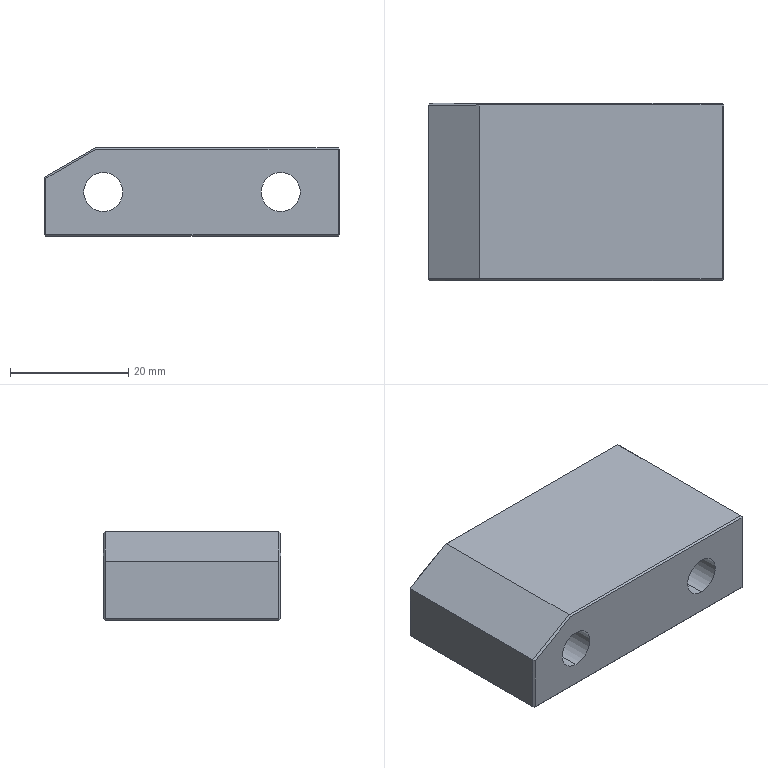Part | SolidWorks | features Chamfer 2, Extrusion 1, HoleWzd 1 | 1 solid | 36 faces | box 50 x 30 x 15 mm | volume 18955 mm3 | plane 28 | cylinder 8 | commonest cylinder face diameters 6.6 x4 11 x4
STEP:
#1=CARTESIAN_POINT('',(-15.,8.2,2.));
#2=VERTEX_POINT('',#1);
#3=CARTESIAN_POINT('',(-15.,8.2,13.));
#4=VERTEX_POINT('',#3);
#5=CARTESIAN_POINT('',(-15.,8.2,7.5));
#6=DIRECTION('',(0.,1.,0.));
#7=DIRECTION('',(0.,0.,1.));
#8=AXIS2_PLACEMENT_3D('',#5,#6,#7);
#9=CIRCLE('',#8,5.5);
#10=EDGE_CURVE('',#2,#4,#9,.T.);
#11=ORIENTED_EDGE('',*,*,#10,.F.);
#12=CARTESIAN_POINT('',(-15.,15.,2.));
#13=VERTEX_POINT('',#12);
#14=CARTESIAN_POINT('',(-15.,15.,2.));
#15=DIRECTION('',(0.,1.,0.));
#16=VECTOR('',#15,1000.);
#17=LINE('',#14,#16);
#18=EDGE_CURVE('',#2,#13,#17,.T.);
#19=ORIENTED_EDGE('',*,*,#18,.T.);
#20=CARTESIAN_POINT('',(-15.,15.,13.));
#21=VERTEX_POINT('',#20);
#22=CARTESIAN_POINT('',(-15.,15.,7.5));
#23=DIRECTION('',(0.,1.,0.));
#24=DIRECTION('',(0.,0.,1.));
#25=AXIS2_PLACEMENT_3D('',#22,#23,#24);
#26=CIRCLE('',#25,5.5);
#27=EDGE_CURVE('',#13,#21,#26,.T.);
#28=ORIENTED_EDGE('',*,*,#27,.T.);
#29=CARTESIAN_POINT('',(-15.,15.,13.));
#30=DIRECTION('',(0.,1.,0.));
#31=VECTOR('',#30,1000.);
#32=LINE('',#29,#31);
#33=EDGE_CURVE('',#4,#21,#32,.T.);
#34=ORIENTED_EDGE('',*,*,#33,.F.);
#35=EDGE_LOOP('',(#11,#19,#28,#34));
#36=FACE_OUTER_BOUND('',#35,.T.);
#37=CARTESIAN_POINT('',(-15.,15.,7.5));
#38=DIRECTION('',(0.,1.,0.));
#39=DIRECTION('',(0.,0.,1.));
#40=AXIS2_PLACEMENT_3D('',#37,#38,#39);
#41=CYLINDRICAL_SURFACE('',#40,5.5);
#42=ADVANCED_FACE('',(#36),#41,.F.);
#43=CARTESIAN_POINT('',(-15.,-15.,4.2));
#44=VERTEX_POINT('',#43);
#45=CARTESIAN_POINT('',(-15.,-15.,10.8));
#46=VERTEX_POINT('',#45);
#47=CARTESIAN_POINT('',(-15.,-15.,7.5));
#48=DIRECTION('',(0.,1.,0.));
#49=DIRECTION('',(0.,0.,1.));
#50=AXIS2_PLACEMENT_3D('',#47,#48,#49);
#51=CIRCLE('',#50,3.3);
#52=EDGE_CURVE('',#44,#46,#51,.T.);
#53=ORIENTED_EDGE('',*,*,#52,.F.);
#54=CARTESIAN_POINT('',(-15.,8.2,4.2));
#55=VERTEX_POINT('',#54);
#56=CARTESIAN_POINT('',(-15.,15.,4.2));
#57=DIRECTION('',(0.,1.,0.));
#58=VECTOR('',#57,1000.);
#59=LINE('',#56,#58);
#60=EDGE_CURVE('',#44,#55,#59,.T.);
#61=ORIENTED_EDGE('',*,*,#60,.T.);
#62=CARTESIAN_POINT('',(-15.,8.2,10.8));
#63=VERTEX_POINT('',#62);
#64=CARTESIAN_POINT('',(-15.,8.2,7.5));
#65=DIRECTION('',(0.,1.,0.));
#66=DIRECTION('',(0.,0.,1.));
#67=AXIS2_PLACEMENT_3D('',#64,#65,#66);
#68=CIRCLE('',#67,3.3);
#69=EDGE_CURVE('',#55,#63,#68,.T.);
#70=ORIENTED_EDGE('',*,*,#69,.T.);
#71=CARTESIAN_POINT('',(-15.,15.,10.8));
#72=DIRECTION('',(0.,1.,0.));
#73=VECTOR('',#72,1000.);
#74=LINE('',#71,#73);
#75=EDGE_CURVE('',#46,#63,#74,.T.);
#76=ORIENTED_EDGE('',*,*,#75,.F.);
#77=EDGE_LOOP('',(#53,#61,#70,#76));
#78=FACE_OUTER_BOUND('',#77,.T.);
#79=CARTESIAN_POINT('',(-15.,15.,7.5));
#80=DIRECTION('',(0.,1.,0.));
#81=DIRECTION('',(0.,0.,1.));
#82=AXIS2_PLACEMENT_3D('',#79,#80,#81);
#83=CYLINDRICAL_SURFACE('',#82,3.3);
#84=ADVANCED_FACE('',(#78),#83,.F.);
#85=CARTESIAN_POINT('',(15.,8.2,2.));
#86=VERTEX_POINT('',#85);
#87=CARTESIAN_POINT('',(15.,8.2,13.));
#88=VERTEX_POINT('',#87);
#89=CARTESIAN_POINT('',(15.,8.2,7.5));
#90=DIRECTION('',(0.,1.,0.));
#91=DIRECTION('',(0.,0.,1.));
#92=AXIS2_PLACEMENT_3D('',#89,#90,#91);
#93=CIRCLE('',#92,5.5);
#94=EDGE_CURVE('',#86,#88,#93,.T.);
#95=ORIENTED_EDGE('',*,*,#94,.F.);
#96=CARTESIAN_POINT('',(15.,15.,2.));
#97=VERTEX_POINT('',#96);
#98=CARTESIAN_POINT('',(15.,15.,2.));
#99=DIRECTION('',(0.,1.,0.));
#100=VECTOR('',#99,1000.);
#101=LINE('',#98,#100);
#102=EDGE_CURVE('',#86,#97,#101,.T.);
#103=ORIENTED_EDGE('',*,*,#102,.T.);
#104=CARTESIAN_POINT('',(15.,15.,13.));
#105=VERTEX_POINT('',#104);
#106=CARTESIAN_POINT('',(15.,15.,7.5));
#107=DIRECTION('',(0.,1.,0.));
#108=DIRECTION('',(0.,0.,1.));
#109=AXIS2_PLACEMENT_3D('',#106,#107,#108);
#110=CIRCLE('',#109,5.5);
#111=EDGE_CURVE('',#97,#105,#110,.T.);
#112=ORIENTED_EDGE('',*,*,#111,.T.);
#113=CARTESIAN_POINT('',(15.,15.,13.));
#114=DIRECTION('',(0.,1.,0.));
#115=VECTOR('',#114,1000.);
#116=LINE('',#113,#115);
#117=EDGE_CURVE('',#88,#105,#116,.T.);
#118=ORIENTED_EDGE('',*,*,#117,.F.);
#119=EDGE_LOOP('',(#95,#103,#112,#118));
#120=FACE_OUTER_BOUND('',#119,.T.);
#121=CARTESIAN_POINT('',(15.,15.,7.5));
#122=DIRECTION('',(0.,1.,0.));
#123=DIRECTION('',(0.,0.,1.));
#124=AXIS2_PLACEMENT_3D('',#121,#122,#123);
#125=CYLINDRICAL_SURFACE('',#124,5.5);
#126=ADVANCED_FACE('',(#120),#125,.F.);
#127=CARTESIAN_POINT('',(15.,-15.,4.2));
#128=VERTEX_POINT('',#127);
#129=CARTESIAN_POINT('',(15.,-15.,10.8));
#130=VERTEX_POINT('',#129);
#131=CARTESIAN_POINT('',(15.,-15.,7.5));
#132=DIRECTION('',(0.,1.,0.));
#133=DIRECTION('',(0.,0.,1.));
#134=AXIS2_PLACEMENT_3D('',#131,#132,#133);
#135=CIRCLE('',#134,3.3);
#136=EDGE_CURVE('',#128,#130,#135,.T.);
#137=ORIENTED_EDGE('',*,*,#136,.F.);
#138=CARTESIAN_POINT('',(15.,8.2,4.2));
#139=VERTEX_POINT('',#138);
#140=CARTESIAN_POINT('',(15.,15.,4.2));
#141=DIRECTION('',(0.,1.,0.));
#142=VECTOR('',#141,1000.);
#143=LINE('',#140,#142);
#144=EDGE_CURVE('',#128,#139,#143,.T.);
#145=ORIENTED_EDGE('',*,*,#144,.T.);
#146=CARTESIAN_POINT('',(15.,8.2,10.8));
#147=VERTEX_POINT('',#146);
#148=CARTESIAN_POINT('',(15.,8.2,7.5));
#149=DIRECTION('',(0.,1.,0.));
#150=DIRECTION('',(0.,0.,1.));
#151=AXIS2_PLACEMENT_3D('',#148,#149,#150);
#152=CIRCLE('',#151,3.3);
#153=EDGE_CURVE('',#139,#147,#152,.T.);
#154=ORIENTED_EDGE('',*,*,#153,.T.);
#155=CARTESIAN_POINT('',(15.,15.,10.8));
#156=DIRECTION('',(0.,1.,0.));
#157=VECTOR('',#156,1000.);
#158=LINE('',#155,#157);
#159=EDGE_CURVE('',#130,#147,#158,.T.);
#160=ORIENTED_EDGE('',*,*,#159,.F.);
#161=EDGE_LOOP('',(#137,#145,#154,#160));
#162=FACE_OUTER_BOUND('',#161,.T.);
#163=CARTESIAN_POINT('',(15.,15.,7.5));
#164=DIRECTION('',(0.,1.,0.));
#165=DIRECTION('',(0.,0.,1.));
#166=AXIS2_PLACEMENT_3D('',#163,#164,#165);
#167=CYLINDRICAL_SURFACE('',#166,3.3);
#168=ADVANCED_FACE('',(#162),#167,.F.);
#169=CARTESIAN_POINT('',(25.,14.7,14.7));
#170=VERTEX_POINT('',#169);
#171=CARTESIAN_POINT('',(25.,-14.7,14.7));
#172=VERTEX_POINT('',#171);
#173=CARTESIAN_POINT('',(25.,-15.,14.7));
#174=DIRECTION('',(0.,-1.,0.));
#175=VECTOR('',#174,1000.);
#176=LINE('',#173,#175);
#177=EDGE_CURVE('',#170,#172,#176,.T.);
#178=ORIENTED_EDGE('',*,*,#177,.T.);
#179=CARTESIAN_POINT('',(25.,-14.7,0.3));
#180=VERTEX_POINT('',#179);
#181=CARTESIAN_POINT('',(25.,-14.7,15.));
#182=DIRECTION('',(0.,0.,-1.));
#183=VECTOR('',#182,1000.);
#184=LINE('',#181,#183);
#185=EDGE_CURVE('',#172,#180,#184,.T.);
#186=ORIENTED_EDGE('',*,*,#185,.T.);
#187=CARTESIAN_POINT('',(25.,14.7,0.3));
#188=VERTEX_POINT('',#187);
#189=CARTESIAN_POINT('',(25.,15.,0.3));
#190=DIRECTION('',(0.,1.,0.));
#191=VECTOR('',#190,1000.);
#192=LINE('',#189,#191);
#193=EDGE_CURVE('',#180,#188,#192,.T.);
#194=ORIENTED_EDGE('',*,*,#193,.T.);
#195=CARTESIAN_POINT('',(25.,14.7,15.));
#196=DIRECTION('',(0.,0.,1.));
#197=VECTOR('',#196,1000.);
#198=LINE('',#195,#197);
#199=EDGE_CURVE('',#188,#170,#198,.T.);
#200=ORIENTED_EDGE('',*,*,#199,.T.);
#201=EDGE_LOOP('',(#178,#186,#194,#200));
#202=FACE_OUTER_BOUND('',#201,.T.);
#203=CARTESIAN_POINT('',(25.,15.,15.));
#204=DIRECTION('',(-1.,0.,0.));
#205=DIRECTION('',(0.,-1.,0.));
#206=AXIS2_PLACEMENT_3D('',#203,#204,#205);
#207=PLANE('',#206);
#208=ADVANCED_FACE('',(#202),#207,.F.);
#209=CARTESIAN_POINT('',(-16.259,15.,14.7));
#210=VERTEX_POINT('',#209);
#211=CARTESIAN_POINT('',(24.7,15.,14.7));
#212=VERTEX_POINT('',#211);
#213=CARTESIAN_POINT('',(25.,15.,14.7));
#214=DIRECTION('',(1.,0.,0.));
#215=VECTOR('',#214,1000.);
#216=LINE('',#213,#215);
#217=EDGE_CURVE('',#210,#212,#216,.T.);
#218=ORIENTED_EDGE('',*,*,#217,.T.);
#219=CARTESIAN_POINT('',(24.7,15.,0.3));
#220=VERTEX_POINT('',#219);
#221=CARTESIAN_POINT('',(24.7,15.,15.));
#222=DIRECTION('',(0.,0.,-1.));
#223=VECTOR('',#222,1000.);
#224=LINE('',#221,#223);
#225=EDGE_CURVE('',#212,#220,#224,.T.);
#226=ORIENTED_EDGE('',*,*,#225,.T.);
#227=CARTESIAN_POINT('',(-24.7,15.,0.3));
#228=VERTEX_POINT('',#227);
#229=CARTESIAN_POINT('',(-25.,15.,0.3));
#230=DIRECTION('',(-1.,0.,0.));
#231=VECTOR('',#230,1000.);
#232=LINE('',#229,#231);
#233=EDGE_CURVE('',#220,#228,#232,.T.);
#234=ORIENTED_EDGE('',*,*,#233,.T.);
#235=CARTESIAN_POINT('',(-24.7,15.,9.827));
#236=VERTEX_POINT('',#235);
#237=CARTESIAN_POINT('',(-24.7,15.,15.));
#238=DIRECTION('',(0.,0.,1.));
#239=VECTOR('',#238,1000.);
#240=LINE('',#237,#239);
#241=EDGE_CURVE('',#228,#236,#240,.T.);
#242=ORIENTED_EDGE('',*,*,#241,.T.);
#243=CARTESIAN_POINT('',(-16.19,15.,14.74));
#244=DIRECTION('',(0.866,0.,0.5));
#245=VECTOR('',#244,1000.);
#246=LINE('',#243,#245);
#247=EDGE_CURVE('',#236,#210,#246,.T.);
#248=ORIENTED_EDGE('',*,*,#247,.T.);
#249=EDGE_LOOP('',(#218,#226,#234,#242,#248));
#250=FACE_OUTER_BOUND('',#249,.T.);
#251=CARTESIAN_POINT('',(-15.,15.,7.5));
#252=DIRECTION('',(0.,1.,0.));
#253=DIRECTION('',(0.,0.,1.));
#254=AXIS2_PLACEMENT_3D('',#251,#252,#253);
#255=CIRCLE('',#254,5.5);
#256=EDGE_CURVE('',#21,#13,#255,.T.);
#257=ORIENTED_EDGE('',*,*,#256,.F.);
#258=ORIENTED_EDGE('',*,*,#27,.F.);
#259=EDGE_LOOP('',(#257,#258));
#260=FACE_BOUND('',#259,.T.);
#261=CARTESIAN_POINT('',(15.,15.,7.5));
#262=DIRECTION('',(0.,1.,0.));
#263=DIRECTION('',(0.,0.,1.));
#264=AXIS2_PLACEMENT_3D('',#261,#262,#263);
#265=CIRCLE('',#264,5.5);
#266=EDGE_CURVE('',#105,#97,#265,.T.);
#267=ORIENTED_EDGE('',*,*,#266,.F.);
#268=ORIENTED_EDGE('',*,*,#111,.F.);
#269=EDGE_LOOP('',(#267,#268));
#270=FACE_BOUND('',#269,.T.);
#271=CARTESIAN_POINT('',(-25.,15.,15.));
#272=DIRECTION('',(0.,-1.,0.));
#273=DIRECTION('',(0.,0.,-1.));
#274=AXIS2_PLACEMENT_3D('',#271,#272,#273);
#275=PLANE('',#274);
#276=ADVANCED_FACE('',(#250,#260,#270),#275,.F.);
#277=CARTESIAN_POINT('',(-25.,-14.7,10.));
#278=VERTEX_POINT('',#277);
#279=CARTESIAN_POINT('',(-25.,14.7,10.));
#280=VERTEX_POINT('',#279);
#281=CARTESIAN_POINT('',(-25.,15.,10.));
#282=DIRECTION('',(0.,1.,0.));
#283=VECTOR('',#282,1000.);
#284=LINE('',#281,#283);
#285=EDGE_CURVE('',#278,#280,#284,.T.);
#286=ORIENTED_EDGE('',*,*,#285,.T.);
#287=CARTESIAN_POINT('',(-25.,14.7,0.3));
#288=VERTEX_POINT('',#287);
#289=CARTESIAN_POINT('',(-25.,14.7,15.));
#290=DIRECTION('',(0.,0.,-1.));
#291=VECTOR('',#290,1000.);
#292=LINE('',#289,#291);
#293=EDGE_CURVE('',#280,#288,#292,.T.);
#294=ORIENTED_EDGE('',*,*,#293,.T.);
#295=CARTESIAN_POINT('',(-25.,-14.7,0.3));
#296=VERTEX_POINT('',#295);
#297=CARTESIAN_POINT('',(-25.,15.,0.3));
#298=DIRECTION('',(0.,-1.,0.));
#299=VECTOR('',#298,1000.);
#300=LINE('',#297,#299);
#301=EDGE_CURVE('',#288,#296,#300,.T.);
#302=ORIENTED_EDGE('',*,*,#301,.T.);
#303=CARTESIAN_POINT('',(-25.,-14.7,15.));
#304=DIRECTION('',(0.,0.,1.));
#305=VECTOR('',#304,1000.);
#306=LINE('',#303,#305);
#307=EDGE_CURVE('',#296,#278,#306,.T.);
#308=ORIENTED_EDGE('',*,*,#307,.T.);
#309=EDGE_LOOP('',(#286,#294,#302,#308));
#310=FACE_OUTER_BOUND('',#309,.T.);
#311=CARTESIAN_POINT('',(-25.,15.,15.));
#312=DIRECTION('',(1.,0.,0.));
#313=DIRECTION('',(0.,0.,-1.));
#314=AXIS2_PLACEMENT_3D('',#311,#312,#313);
#315=PLANE('',#314);
#316=ADVANCED_FACE('',(#310),#315,.F.);
#317=CARTESIAN_POINT('',(-24.7,-15.,0.3));
#318=VERTEX_POINT('',#317);
#319=CARTESIAN_POINT('',(24.7,-15.,0.3));
#320=VERTEX_POINT('',#319);
#321=CARTESIAN_POINT('',(-25.,-15.,0.3));
#322=DIRECTION('',(1.,0.,0.));
#323=VECTOR('',#322,1000.);
#324=LINE('',#321,#323);
#325=EDGE_CURVE('',#318,#320,#324,.T.);
#326=ORIENTED_EDGE('',*,*,#325,.T.);
#327=CARTESIAN_POINT('',(24.7,-15.,14.7));
#328=VERTEX_POINT('',#327);
#329=CARTESIAN_POINT('',(24.7,-15.,15.));
#330=DIRECTION('',(0.,0.,1.));
#331=VECTOR('',#330,1000.);
#332=LINE('',#329,#331);
#333=EDGE_CURVE('',#320,#328,#332,.T.);
#334=ORIENTED_EDGE('',*,*,#333,.T.);
#335=CARTESIAN_POINT('',(-16.259,-15.,14.7));
#336=VERTEX_POINT('',#335);
#337=CARTESIAN_POINT('',(-16.34,-15.,14.7));
#338=DIRECTION('',(-1.,0.,0.));
#339=VECTOR('',#338,1000.);
#340=LINE('',#337,#339);
#341=EDGE_CURVE('',#328,#336,#340,.T.);
#342=ORIENTED_EDGE('',*,*,#341,.T.);
#343=CARTESIAN_POINT('',(-24.7,-15.,9.827));
#344=VERTEX_POINT('',#343);
#345=CARTESIAN_POINT('',(-24.85,-15.,9.74));
#346=DIRECTION('',(-0.866,0.,-0.5));
#347=VECTOR('',#346,1000.);
#348=LINE('',#345,#347);
#349=EDGE_CURVE('',#336,#344,#348,.T.);
#350=ORIENTED_EDGE('',*,*,#349,.T.);
#351=CARTESIAN_POINT('',(-24.7,-15.,15.));
#352=DIRECTION('',(0.,0.,-1.));
#353=VECTOR('',#352,1000.);
#354=LINE('',#351,#353);
#355=EDGE_CURVE('',#344,#318,#354,.T.);
#356=ORIENTED_EDGE('',*,*,#355,.T.);
#357=EDGE_LOOP('',(#326,#334,#342,#350,#356));
#358=FACE_OUTER_BOUND('',#357,.T.);
#359=CARTESIAN_POINT('',(-15.,-15.,7.5));
#360=DIRECTION('',(0.,1.,0.));
#361=DIRECTION('',(0.,0.,1.));
#362=AXIS2_PLACEMENT_3D('',#359,#360,#361);
#363=CIRCLE('',#362,3.3);
#364=EDGE_CURVE('',#46,#44,#363,.T.);
#365=ORIENTED_EDGE('',*,*,#364,.T.);
#366=ORIENTED_EDGE('',*,*,#52,.T.);
#367=EDGE_LOOP('',(#365,#366));
#368=FACE_BOUND('',#367,.T.);
#369=CARTESIAN_POINT('',(15.,-15.,7.5));
#370=DIRECTION('',(0.,1.,0.));
#371=DIRECTION('',(0.,0.,1.));
#372=AXIS2_PLACEMENT_3D('',#369,#370,#371);
#373=CIRCLE('',#372,3.3);
#374=EDGE_CURVE('',#130,#128,#373,.T.);
#375=ORIENTED_EDGE('',*,*,#374,.T.);
#376=ORIENTED_EDGE('',*,*,#136,.T.);
#377=EDGE_LOOP('',(#375,#376));
#378=FACE_BOUND('',#377,.T.);
#379=CARTESIAN_POINT('',(-25.,-15.,15.));
#380=DIRECTION('',(0.,1.,0.));
#381=DIRECTION('',(0.,0.,1.));
#382=AXIS2_PLACEMENT_3D('',#379,#380,#381);
#383=PLANE('',#382);
#384=ADVANCED_FACE('',(#358,#368,#378),#383,.F.);
#385=CARTESIAN_POINT('',(24.7,-14.7,15.));
#386=VERTEX_POINT('',#385);
#387=CARTESIAN_POINT('',(24.7,14.7,15.));
#388=VERTEX_POINT('',#387);
#389=CARTESIAN_POINT('',(24.7,15.,15.));
#390=DIRECTION('',(0.,1.,0.));
#391=VECTOR('',#390,1000.);
#392=LINE('',#389,#391);
#393=EDGE_CURVE('',#386,#388,#392,.T.);
#394=ORIENTED_EDGE('',*,*,#393,.T.);
#395=CARTESIAN_POINT('',(-16.34,14.7,15.));
#396=VERTEX_POINT('',#395);
#397=CARTESIAN_POINT('',(-16.34,14.7,15.));
#398=DIRECTION('',(-1.,0.,0.));
#399=VECTOR('',#398,1000.);
#400=LINE('',#397,#399);
#401=EDGE_CURVE('',#388,#396,#400,.T.);
#402=ORIENTED_EDGE('',*,*,#401,.T.);
#403=CARTESIAN_POINT('',(-16.34,-14.7,15.));
#404=VERTEX_POINT('',#403);
#405=CARTESIAN_POINT('',(-16.34,-15.,15.));
#406=DIRECTION('',(0.,-1.,0.));
#407=VECTOR('',#406,1000.);
#408=LINE('',#405,#407);
#409=EDGE_CURVE('',#396,#404,#408,.T.);
#410=ORIENTED_EDGE('',*,*,#409,.T.);
#411=CARTESIAN_POINT('',(25.,-14.7,15.));
#412=DIRECTION('',(1.,0.,0.));
#413=VECTOR('',#412,1000.);
#414=LINE('',#411,#413);
#415=EDGE_CURVE('',#404,#386,#414,.T.);
#416=ORIENTED_EDGE('',*,*,#415,.T.);
#417=EDGE_LOOP('',(#394,#402,#410,#416));
#418=FACE_OUTER_BOUND('',#417,.T.);
#419=CARTESIAN_POINT('',(0.,0.,15.));
#420=DIRECTION('',(0.,0.,1.));
#421=DIRECTION('',(1.,0.,0.));
#422=AXIS2_PLACEMENT_3D('',#419,#420,#421);
#423=PLANE('',#422);
#424=ADVANCED_FACE('',(#418),#423,.T.);
#425=CARTESIAN_POINT('',(-24.7,-14.7,0.));
#426=VERTEX_POINT('',#425);
#427=CARTESIAN_POINT('',(-24.7,14.7,0.));
#428=VERTEX_POINT('',#427);
#429=CARTESIAN_POINT('',(-24.7,0.,0.));
#430=DIRECTION('',(0.,1.,0.));
#431=VECTOR('',#430,1000.);
#432=LINE('',#429,#431);
#433=EDGE_CURVE('',#426,#428,#432,.T.);
#434=ORIENTED_EDGE('',*,*,#433,.T.);
#435=CARTESIAN_POINT('',(24.7,14.7,0.));
#436=VERTEX_POINT('',#435);
#437=CARTESIAN_POINT('',(0.,14.7,0.));
#438=DIRECTION('',(1.,0.,0.));
#439=VECTOR('',#438,1000.);
#440=LINE('',#437,#439);
#441=EDGE_CURVE('',#428,#436,#440,.T.);
#442=ORIENTED_EDGE('',*,*,#441,.T.);
#443=CARTESIAN_POINT('',(24.7,-14.7,0.));
#444=VERTEX_POINT('',#443);
#445=CARTESIAN_POINT('',(24.7,0.,0.));
#446=DIRECTION('',(0.,-1.,0.));
#447=VECTOR('',#446,1000.);
#448=LINE('',#445,#447);
#449=EDGE_CURVE('',#436,#444,#448,.T.);
#450=ORIENTED_EDGE('',*,*,#449,.T.);
#451=CARTESIAN_POINT('',(0.,-14.7,0.));
#452=DIRECTION('',(-1.,0.,0.));
#453=VECTOR('',#452,1000.);
#454=LINE('',#451,#453);
#455=EDGE_CURVE('',#444,#426,#454,.T.);
#456=ORIENTED_EDGE('',*,*,#455,.T.);
#457=EDGE_LOOP('',(#434,#442,#450,#456));
#458=FACE_OUTER_BOUND('',#457,.T.);
#459=CARTESIAN_POINT('',(0.,0.,0.));
#460=DIRECTION('',(0.,0.,1.));
#461=DIRECTION('',(1.,0.,0.));
#462=AXIS2_PLACEMENT_3D('',#459,#460,#461);
#463=PLANE('',#462);
#464=ADVANCED_FACE('',(#458),#463,.F.);
#465=ORIENTED_EDGE('',*,*,#144,.F.);
#466=ORIENTED_EDGE('',*,*,#374,.F.);
#467=ORIENTED_EDGE('',*,*,#159,.T.);
#468=CARTESIAN_POINT('',(15.,8.2,7.5));
#469=DIRECTION('',(0.,1.,0.));
#470=DIRECTION('',(0.,0.,1.));
#471=AXIS2_PLACEMENT_3D('',#468,#469,#470);
#472=CIRCLE('',#471,3.3);
#473=EDGE_CURVE('',#147,#139,#472,.T.);
#474=ORIENTED_EDGE('',*,*,#473,.T.);
#475=EDGE_LOOP('',(#465,#466,#467,#474));
#476=FACE_OUTER_BOUND('',#475,.T.);
#477=CARTESIAN_POINT('',(15.,15.,7.5));
#478=DIRECTION('',(0.,1.,0.));
#479=DIRECTION('',(0.,0.,1.));
#480=AXIS2_PLACEMENT_3D('',#477,#478,#479);
#481=CYLINDRICAL_SURFACE('',#480,3.3);
#482=ADVANCED_FACE('',(#476),#481,.F.);
#483=ORIENTED_EDGE('',*,*,#473,.F.);
#484=ORIENTED_EDGE('',*,*,#153,.F.);
#485=EDGE_LOOP('',(#483,#484));
#486=FACE_BOUND('',#485,.T.);
#487=CARTESIAN_POINT('',(15.,8.2,7.5));
#488=DIRECTION('',(0.,1.,0.));
#489=DIRECTION('',(0.,0.,1.));
#490=AXIS2_PLACEMENT_3D('',#487,#488,#489);
#491=CIRCLE('',#490,5.5);
#492=EDGE_CURVE('',#88,#86,#491,.T.);
#493=ORIENTED_EDGE('',*,*,#492,.T.);
#494=ORIENTED_EDGE('',*,*,#94,.T.);
#495=EDGE_LOOP('',(#493,#494));
#496=FACE_OUTER_BOUND('',#495,.T.);
#497=CARTESIAN_POINT('',(18.3,8.2,7.5));
#498=DIRECTION('',(0.,-1.,0.));
#499=DIRECTION('',(0.,0.,-1.));
#500=AXIS2_PLACEMENT_3D('',#497,#498,#499);
#501=PLANE('',#500);
#502=ADVANCED_FACE('',(#486,#496),#501,.F.);
#503=ORIENTED_EDGE('',*,*,#102,.F.);
#504=ORIENTED_EDGE('',*,*,#492,.F.);
#505=ORIENTED_EDGE('',*,*,#117,.T.);
#506=ORIENTED_EDGE('',*,*,#266,.T.);
#507=EDGE_LOOP('',(#503,#504,#505,#506));
#508=FACE_OUTER_BOUND('',#507,.T.);
#509=CARTESIAN_POINT('',(15.,15.,7.5));
#510=DIRECTION('',(0.,1.,0.));
#511=DIRECTION('',(0.,0.,1.));
#512=AXIS2_PLACEMENT_3D('',#509,#510,#511);
#513=CYLINDRICAL_SURFACE('',#512,5.5);
#514=ADVANCED_FACE('',(#508),#513,.F.);
#515=ORIENTED_EDGE('',*,*,#60,.F.);
#516=ORIENTED_EDGE('',*,*,#364,.F.);
#517=ORIENTED_EDGE('',*,*,#75,.T.);
#518=CARTESIAN_POINT('',(-15.,8.2,7.5));
#519=DIRECTION('',(0.,1.,0.));
#520=DIRECTION('',(0.,0.,1.));
#521=AXIS2_PLACEMENT_3D('',#518,#519,#520);
#522=CIRCLE('',#521,3.3);
#523=EDGE_CURVE('',#63,#55,#522,.T.);
#524=ORIENTED_EDGE('',*,*,#523,.T.);
#525=EDGE_LOOP('',(#515,#516,#517,#524));
#526=FACE_OUTER_BOUND('',#525,.T.);
#527=CARTESIAN_POINT('',(-15.,15.,7.5));
#528=DIRECTION('',(0.,1.,0.));
#529=DIRECTION('',(0.,0.,1.));
#530=AXIS2_PLACEMENT_3D('',#527,#528,#529);
#531=CYLINDRICAL_SURFACE('',#530,3.3);
#532=ADVANCED_FACE('',(#526),#531,.F.);
#533=ORIENTED_EDGE('',*,*,#523,.F.);
#534=ORIENTED_EDGE('',*,*,#69,.F.);
#535=EDGE_LOOP('',(#533,#534));
#536=FACE_BOUND('',#535,.T.);
#537=CARTESIAN_POINT('',(-15.,8.2,7.5));
#538=DIRECTION('',(0.,1.,0.));
#539=DIRECTION('',(0.,0.,1.));
#540=AXIS2_PLACEMENT_3D('',#537,#538,#539);
#541=CIRCLE('',#540,5.5);
#542=EDGE_CURVE('',#4,#2,#541,.T.);
#543=ORIENTED_EDGE('',*,*,#542,.T.);
#544=ORIENTED_EDGE('',*,*,#10,.T.);
#545=EDGE_LOOP('',(#543,#544));
#546=FACE_OUTER_BOUND('',#545,.T.);
#547=CARTESIAN_POINT('',(-11.7,8.2,7.5));
#548=DIRECTION('',(0.,-1.,0.));
#549=DIRECTION('',(0.,0.,-1.));
#550=AXIS2_PLACEMENT_3D('',#547,#548,#549);
#551=PLANE('',#550);
#552=ADVANCED_FACE('',(#536,#546),#551,.F.);
#553=ORIENTED_EDGE('',*,*,#18,.F.);
#554=ORIENTED_EDGE('',*,*,#542,.F.);
#555=ORIENTED_EDGE('',*,*,#33,.T.);
#556=ORIENTED_EDGE('',*,*,#256,.T.);
#557=EDGE_LOOP('',(#553,#554,#555,#556));
#558=FACE_OUTER_BOUND('',#557,.T.);
#559=CARTESIAN_POINT('',(-15.,15.,7.5));
#560=DIRECTION('',(0.,1.,0.));
#561=DIRECTION('',(0.,0.,1.));
#562=AXIS2_PLACEMENT_3D('',#559,#560,#561);
#563=CYLINDRICAL_SURFACE('',#562,5.5);
#564=ADVANCED_FACE('',(#558),#563,.F.);
#565=ORIENTED_EDGE('',*,*,#409,.F.);
#566=CARTESIAN_POINT('',(-25.,14.7,10.));
#567=DIRECTION('',(-0.866,0.,-0.5));
#568=VECTOR('',#567,1000.);
#569=LINE('',#566,#568);
#570=EDGE_CURVE('',#396,#280,#569,.T.);
#571=ORIENTED_EDGE('',*,*,#570,.T.);
#572=ORIENTED_EDGE('',*,*,#285,.F.);
#573=CARTESIAN_POINT('',(-16.34,-14.7,15.));
#574=DIRECTION('',(0.866,0.,0.5));
#575=VECTOR('',#574,1000.);
#576=LINE('',#573,#575);
#577=EDGE_CURVE('',#278,#404,#576,.T.);
#578=ORIENTED_EDGE('',*,*,#577,.T.);
#579=EDGE_LOOP('',(#565,#571,#572,#578));
#580=FACE_OUTER_BOUND('',#579,.T.);
#581=CARTESIAN_POINT('',(-16.34,0.,15.));
#582=DIRECTION('',(-0.5,0.,0.866));
#583=DIRECTION('',(0.,1.,0.));
#584=AXIS2_PLACEMENT_3D('',#581,#582,#583);
#585=PLANE('',#584);
#586=ADVANCED_FACE('',(#580),#585,.T.);
#587=CARTESIAN_POINT('',(-24.7,15.,0.3));
#588=DIRECTION('',(0.7071,0.7071,0.));
#589=VECTOR('',#588,1000.);
#590=LINE('',#587,#589);
#591=EDGE_CURVE('',#288,#228,#590,.T.);
#592=ORIENTED_EDGE('',*,*,#591,.F.);
#593=ORIENTED_EDGE('',*,*,#293,.F.);
#594=CARTESIAN_POINT('',(-26.237,13.463,10.714));
#595=DIRECTION('',(-0.6547,-0.6547,0.378));
#596=VECTOR('',#595,1000.);
#597=LINE('',#594,#596);
#598=EDGE_CURVE('',#236,#280,#597,.T.);
#599=ORIENTED_EDGE('',*,*,#598,.F.);
#600=ORIENTED_EDGE('',*,*,#241,.F.);
#601=EDGE_LOOP('',(#592,#593,#599,#600));
#602=FACE_OUTER_BOUND('',#601,.T.);
#603=CARTESIAN_POINT('',(-25.,14.7,15.));
#604=DIRECTION('',(0.7071,-0.7071,0.));
#605=DIRECTION('',(0.,0.,-1.));
#606=AXIS2_PLACEMENT_3D('',#603,#604,#605);
#607=PLANE('',#606);
#608=ADVANCED_FACE('',(#602),#607,.F.);
#609=ORIENTED_EDGE('',*,*,#598,.T.);
#610=ORIENTED_EDGE('',*,*,#570,.F.);
#611=CARTESIAN_POINT('',(-16.002,15.96,13.74));
#612=DIRECTION('',(-0.1862,-0.6947,0.6947));
#613=VECTOR('',#612,1000.);
#614=LINE('',#611,#613);
#615=EDGE_CURVE('',#210,#396,#614,.T.);
#616=ORIENTED_EDGE('',*,*,#615,.F.);
#617=ORIENTED_EDGE('',*,*,#247,.F.);
#618=EDGE_LOOP('',(#609,#610,#616,#617));
#619=FACE_OUTER_BOUND('',#618,.T.);
#620=CARTESIAN_POINT('',(-22.685,15.,10.99));
#621=DIRECTION('',(-0.3536,0.7071,0.6124));
#622=DIRECTION('',(-0.866,0.,-0.5));
#623=AXIS2_PLACEMENT_3D('',#620,#621,#622);
#624=PLANE('',#623);
#625=ADVANCED_FACE('',(#619),#624,.T.);
#626=CARTESIAN_POINT('',(-24.85,14.7,0.15));
#627=DIRECTION('',(0.7071,0.,-0.7071));
#628=VECTOR('',#627,1000.);
#629=LINE('',#626,#628);
#630=EDGE_CURVE('',#288,#428,#629,.T.);
#631=ORIENTED_EDGE('',*,*,#630,.F.);
#632=ORIENTED_EDGE('',*,*,#591,.T.);
#633=CARTESIAN_POINT('',(-24.7,15.,0.3));
#634=DIRECTION('',(0.,0.7071,0.7071));
#635=VECTOR('',#634,1000.);
#636=LINE('',#633,#635);
#637=EDGE_CURVE('',#428,#228,#636,.T.);
#638=ORIENTED_EDGE('',*,*,#637,.F.);
#639=EDGE_LOOP('',(#631,#632,#638));
#640=FACE_OUTER_BOUND('',#639,.T.);
#641=CARTESIAN_POINT('',(-24.7,15.,0.3));
#642=DIRECTION('',(-0.5774,0.5774,-0.5774));
#643=DIRECTION('',(-0.7071,0.,0.7071));
#644=AXIS2_PLACEMENT_3D('',#641,#642,#643);
#645=PLANE('',#644);
#646=ADVANCED_FACE('',(#640),#645,.T.);
#647=ORIENTED_EDGE('',*,*,#615,.T.);
#648=ORIENTED_EDGE('',*,*,#401,.F.);
#649=CARTESIAN_POINT('',(24.7,14.7,15.));
#650=DIRECTION('',(0.,-0.7071,0.7071));
#651=VECTOR('',#650,1000.);
#652=LINE('',#649,#651);
#653=EDGE_CURVE('',#212,#388,#652,.T.);
#654=ORIENTED_EDGE('',*,*,#653,.F.);
#655=ORIENTED_EDGE('',*,*,#217,.F.);
#656=EDGE_LOOP('',(#647,#648,#654,#655));
#657=FACE_OUTER_BOUND('',#656,.T.);
#658=CARTESIAN_POINT('',(0.,14.7,15.));
#659=DIRECTION('',(0.,0.7071,0.7071));
#660=DIRECTION('',(1.,0.,0.));
#661=AXIS2_PLACEMENT_3D('',#658,#659,#660);
#662=PLANE('',#661);
#663=ADVANCED_FACE('',(#657),#662,.T.);
#664=CARTESIAN_POINT('',(24.7,15.,0.3));
#665=DIRECTION('',(0.7071,-0.7071,0.));
#666=VECTOR('',#665,1000.);
#667=LINE('',#664,#666);
#668=EDGE_CURVE('',#220,#188,#667,.T.);
#669=ORIENTED_EDGE('',*,*,#668,.F.);
#670=ORIENTED_EDGE('',*,*,#225,.F.);
#671=CARTESIAN_POINT('',(24.85,14.85,14.7));
#672=DIRECTION('',(-0.7071,0.7071,0.));
#673=VECTOR('',#672,1000.);
#674=LINE('',#671,#673);
#675=EDGE_CURVE('',#170,#212,#674,.T.);
#676=ORIENTED_EDGE('',*,*,#675,.F.);
#677=ORIENTED_EDGE('',*,*,#199,.F.);
#678=EDGE_LOOP('',(#669,#670,#676,#677));
#679=FACE_OUTER_BOUND('',#678,.T.);
#680=CARTESIAN_POINT('',(24.7,15.,15.));
#681=DIRECTION('',(-0.7071,-0.7071,0.));
#682=DIRECTION('',(0.,0.,-1.));
#683=AXIS2_PLACEMENT_3D('',#680,#681,#682);
#684=PLANE('',#683);
#685=ADVANCED_FACE('',(#679),#684,.F.);
#686=ORIENTED_EDGE('',*,*,#637,.T.);
#687=ORIENTED_EDGE('',*,*,#233,.F.);
#688=CARTESIAN_POINT('',(24.7,15.,0.3));
#689=DIRECTION('',(0.,0.7071,0.7071));
#690=VECTOR('',#689,1000.);
#691=LINE('',#688,#690);
#692=EDGE_CURVE('',#436,#220,#691,.T.);
#693=ORIENTED_EDGE('',*,*,#692,.F.);
#694=ORIENTED_EDGE('',*,*,#441,.F.);
#695=EDGE_LOOP('',(#686,#687,#693,#694));
#696=FACE_OUTER_BOUND('',#695,.T.);
#697=CARTESIAN_POINT('',(-25.,15.,0.3));
#698=DIRECTION('',(0.,-0.7071,0.7071));
#699=DIRECTION('',(-1.,0.,0.));
#700=AXIS2_PLACEMENT_3D('',#697,#698,#699);
#701=PLANE('',#700);
#702=ADVANCED_FACE('',(#696),#701,.F.);
#703=ORIENTED_EDGE('',*,*,#630,.T.);
#704=ORIENTED_EDGE('',*,*,#433,.F.);
#705=CARTESIAN_POINT('',(-25.,-14.7,0.3));
#706=DIRECTION('',(0.7071,0.,-0.7071));
#707=VECTOR('',#706,1000.);
#708=LINE('',#705,#707);
#709=EDGE_CURVE('',#296,#426,#708,.T.);
#710=ORIENTED_EDGE('',*,*,#709,.F.);
#711=ORIENTED_EDGE('',*,*,#301,.F.);
#712=EDGE_LOOP('',(#703,#704,#710,#711));
#713=FACE_OUTER_BOUND('',#712,.T.);
#714=CARTESIAN_POINT('',(-25.,15.,0.3));
#715=DIRECTION('',(0.7071,0.,0.7071));
#716=DIRECTION('',(0.,-1.,0.));
#717=AXIS2_PLACEMENT_3D('',#714,#715,#716);
#718=PLANE('',#717);
#719=ADVANCED_FACE('',(#713),#718,.F.);
#720=CARTESIAN_POINT('',(-25.,-14.7,0.3));
#721=DIRECTION('',(-0.7071,0.7071,0.));
#722=VECTOR('',#721,1000.);
#723=LINE('',#720,#722);
#724=EDGE_CURVE('',#318,#296,#723,.T.);
#725=ORIENTED_EDGE('',*,*,#724,.F.);
#726=ORIENTED_EDGE('',*,*,#355,.F.);
#727=CARTESIAN_POINT('',(-25.98,-13.72,10.566));
#728=DIRECTION('',(0.6547,-0.6547,-0.378));
#729=VECTOR('',#728,1000.);
#730=LINE('',#727,#729);
#731=EDGE_CURVE('',#278,#344,#730,.T.);
#732=ORIENTED_EDGE('',*,*,#731,.F.);
#733=ORIENTED_EDGE('',*,*,#307,.F.);
#734=EDGE_LOOP('',(#725,#726,#732,#733));
#735=FACE_OUTER_BOUND('',#734,.T.);
#736=CARTESIAN_POINT('',(-24.7,-15.,15.));
#737=DIRECTION('',(0.7071,0.7071,0.));
#738=DIRECTION('',(0.,0.,-1.));
#739=AXIS2_PLACEMENT_3D('',#736,#737,#738);
#740=PLANE('',#739);
#741=ADVANCED_FACE('',(#735),#740,.F.);
#742=ORIENTED_EDGE('',*,*,#731,.T.);
#743=ORIENTED_EDGE('',*,*,#349,.F.);
#744=CARTESIAN_POINT('',(-16.002,-15.96,13.74));
#745=DIRECTION('',(0.1862,-0.6947,-0.6947));
#746=VECTOR('',#745,1000.);
#747=LINE('',#744,#746);
#748=EDGE_CURVE('',#404,#336,#747,.T.);
#749=ORIENTED_EDGE('',*,*,#748,.F.);
#750=ORIENTED_EDGE('',*,*,#577,.F.);
#751=EDGE_LOOP('',(#742,#743,#749,#750));
#752=FACE_OUTER_BOUND('',#751,.T.);
#753=CARTESIAN_POINT('',(-22.685,-15.,10.99));
#754=DIRECTION('',(-0.3536,-0.7071,0.6124));
#755=DIRECTION('',(0.866,0.,0.5));
#756=AXIS2_PLACEMENT_3D('',#753,#754,#755);
#757=PLANE('',#756);
#758=ADVANCED_FACE('',(#752),#757,.T.);
#759=ORIENTED_EDGE('',*,*,#675,.T.);
#760=ORIENTED_EDGE('',*,*,#653,.T.);
#761=CARTESIAN_POINT('',(24.7,14.7,15.));
#762=DIRECTION('',(-0.7071,0.,0.7071));
#763=VECTOR('',#762,1000.);
#764=LINE('',#761,#763);
#765=EDGE_CURVE('',#170,#388,#764,.T.);
#766=ORIENTED_EDGE('',*,*,#765,.F.);
#767=EDGE_LOOP('',(#759,#760,#766));
#768=FACE_OUTER_BOUND('',#767,.T.);
#769=CARTESIAN_POINT('',(24.7,14.7,15.));
#770=DIRECTION('',(0.5774,0.5774,0.5774));
#771=DIRECTION('',(-0.7071,0.7071,0.));
#772=AXIS2_PLACEMENT_3D('',#769,#770,#771);
#773=PLANE('',#772);
#774=ADVANCED_FACE('',(#768),#773,.T.);
#775=ORIENTED_EDGE('',*,*,#692,.T.);
#776=ORIENTED_EDGE('',*,*,#668,.T.);
#777=CARTESIAN_POINT('',(24.85,14.7,0.15));
#778=DIRECTION('',(0.7071,0.,0.7071));
#779=VECTOR('',#778,1000.);
#780=LINE('',#777,#779);
#781=EDGE_CURVE('',#436,#188,#780,.T.);
#782=ORIENTED_EDGE('',*,*,#781,.F.);
#783=EDGE_LOOP('',(#775,#776,#782));
#784=FACE_OUTER_BOUND('',#783,.T.);
#785=CARTESIAN_POINT('',(24.7,15.,0.3));
#786=DIRECTION('',(0.5774,0.5774,-0.5774));
#787=DIRECTION('',(-0.7071,0.7071,0.));
#788=AXIS2_PLACEMENT_3D('',#785,#786,#787);
#789=PLANE('',#788);
#790=ADVANCED_FACE('',(#784),#789,.T.);
#791=ORIENTED_EDGE('',*,*,#724,.T.);
#792=ORIENTED_EDGE('',*,*,#709,.T.);
#793=CARTESIAN_POINT('',(-24.7,-14.85,0.15));
#794=DIRECTION('',(0.,0.7071,-0.7071));
#795=VECTOR('',#794,1000.);
#796=LINE('',#793,#795);
#797=EDGE_CURVE('',#318,#426,#796,.T.);
#798=ORIENTED_EDGE('',*,*,#797,.F.);
#799=EDGE_LOOP('',(#791,#792,#798));
#800=FACE_OUTER_BOUND('',#799,.T.);
#801=CARTESIAN_POINT('',(-25.,-14.7,0.3));
#802=DIRECTION('',(-0.5774,-0.5774,-0.5774));
#803=DIRECTION('',(-0.7071,0.,0.7071));
#804=AXIS2_PLACEMENT_3D('',#801,#802,#803);
#805=PLANE('',#804);
#806=ADVANCED_FACE('',(#800),#805,.T.);
#807=ORIENTED_EDGE('',*,*,#748,.T.);
#808=ORIENTED_EDGE('',*,*,#341,.F.);
#809=CARTESIAN_POINT('',(24.7,-15.,14.7));
#810=DIRECTION('',(0.,-0.7071,-0.7071));
#811=VECTOR('',#810,1000.);
#812=LINE('',#809,#811);
#813=EDGE_CURVE('',#386,#328,#812,.T.);
#814=ORIENTED_EDGE('',*,*,#813,.F.);
#815=ORIENTED_EDGE('',*,*,#415,.F.);
#816=EDGE_LOOP('',(#807,#808,#814,#815));
#817=FACE_OUTER_BOUND('',#816,.T.);
#818=CARTESIAN_POINT('',(0.,-14.7,15.));
#819=DIRECTION('',(0.,-0.7071,0.7071));
#820=DIRECTION('',(-1.,0.,0.));
#821=AXIS2_PLACEMENT_3D('',#818,#819,#820);
#822=PLANE('',#821);
#823=ADVANCED_FACE('',(#817),#822,.T.);
#824=ORIENTED_EDGE('',*,*,#765,.T.);
#825=ORIENTED_EDGE('',*,*,#393,.F.);
#826=CARTESIAN_POINT('',(24.85,-14.7,14.85));
#827=DIRECTION('',(-0.7071,0.,0.7071));
#828=VECTOR('',#827,1000.);
#829=LINE('',#826,#828);
#830=EDGE_CURVE('',#172,#386,#829,.T.);
#831=ORIENTED_EDGE('',*,*,#830,.F.);
#832=ORIENTED_EDGE('',*,*,#177,.F.);
#833=EDGE_LOOP('',(#824,#825,#831,#832));
#834=FACE_OUTER_BOUND('',#833,.T.);
#835=CARTESIAN_POINT('',(24.7,0.,15.));
#836=DIRECTION('',(0.7071,0.,0.7071));
#837=DIRECTION('',(0.,-1.,0.));
#838=AXIS2_PLACEMENT_3D('',#835,#836,#837);
#839=PLANE('',#838);
#840=ADVANCED_FACE('',(#834),#839,.T.);
#841=ORIENTED_EDGE('',*,*,#781,.T.);
#842=ORIENTED_EDGE('',*,*,#193,.F.);
#843=CARTESIAN_POINT('',(25.,-14.7,0.3));
#844=DIRECTION('',(0.7071,0.,0.7071));
#845=VECTOR('',#844,1000.);
#846=LINE('',#843,#845);
#847=EDGE_CURVE('',#444,#180,#846,.T.);
#848=ORIENTED_EDGE('',*,*,#847,.F.);
#849=ORIENTED_EDGE('',*,*,#449,.F.);
#850=EDGE_LOOP('',(#841,#842,#848,#849));
#851=FACE_OUTER_BOUND('',#850,.T.);
#852=CARTESIAN_POINT('',(25.,15.,0.3));
#853=DIRECTION('',(-0.7071,0.,0.7071));
#854=DIRECTION('',(0.,1.,0.));
#855=AXIS2_PLACEMENT_3D('',#852,#853,#854);
#856=PLANE('',#855);
#857=ADVANCED_FACE('',(#851),#856,.F.);
#858=ORIENTED_EDGE('',*,*,#797,.T.);
#859=ORIENTED_EDGE('',*,*,#455,.F.);
#860=CARTESIAN_POINT('',(24.7,-14.85,0.15));
#861=DIRECTION('',(0.,0.7071,-0.7071));
#862=VECTOR('',#861,1000.);
#863=LINE('',#860,#862);
#864=EDGE_CURVE('',#320,#444,#863,.T.);
#865=ORIENTED_EDGE('',*,*,#864,.F.);
#866=ORIENTED_EDGE('',*,*,#325,.F.);
#867=EDGE_LOOP('',(#858,#859,#865,#866));
#868=FACE_OUTER_BOUND('',#867,.T.);
#869=CARTESIAN_POINT('',(-25.,-15.,0.3));
#870=DIRECTION('',(0.,0.7071,0.7071));
#871=DIRECTION('',(1.,0.,0.));
#872=AXIS2_PLACEMENT_3D('',#869,#870,#871);
#873=PLANE('',#872);
#874=ADVANCED_FACE('',(#868),#873,.F.);
#875=ORIENTED_EDGE('',*,*,#830,.T.);
#876=ORIENTED_EDGE('',*,*,#813,.T.);
#877=CARTESIAN_POINT('',(24.7,-15.,14.7));
#878=DIRECTION('',(-0.7071,-0.7071,0.));
#879=VECTOR('',#878,1000.);
#880=LINE('',#877,#879);
#881=EDGE_CURVE('',#172,#328,#880,.T.);
#882=ORIENTED_EDGE('',*,*,#881,.F.);
#883=EDGE_LOOP('',(#875,#876,#882));
#884=FACE_OUTER_BOUND('',#883,.T.);
#885=CARTESIAN_POINT('',(24.7,-15.,14.7));
#886=DIRECTION('',(0.5774,-0.5774,0.5774));
#887=DIRECTION('',(0.7071,0.7071,0.));
#888=AXIS2_PLACEMENT_3D('',#885,#886,#887);
#889=PLANE('',#888);
#890=ADVANCED_FACE('',(#884),#889,.T.);
#891=ORIENTED_EDGE('',*,*,#864,.T.);
#892=ORIENTED_EDGE('',*,*,#847,.T.);
#893=CARTESIAN_POINT('',(25.,-14.7,0.3));
#894=DIRECTION('',(0.7071,0.7071,0.));
#895=VECTOR('',#894,1000.);
#896=LINE('',#893,#895);
#897=EDGE_CURVE('',#320,#180,#896,.T.);
#898=ORIENTED_EDGE('',*,*,#897,.F.);
#899=EDGE_LOOP('',(#891,#892,#898));
#900=FACE_OUTER_BOUND('',#899,.T.);
#901=CARTESIAN_POINT('',(25.,-14.7,0.3));
#902=DIRECTION('',(0.5774,-0.5774,-0.5774));
#903=DIRECTION('',(0.7071,0.7071,0.));
#904=AXIS2_PLACEMENT_3D('',#901,#902,#903);
#905=PLANE('',#904);
#906=ADVANCED_FACE('',(#900),#905,.T.);
#907=ORIENTED_EDGE('',*,*,#881,.T.);
#908=ORIENTED_EDGE('',*,*,#333,.F.);
#909=ORIENTED_EDGE('',*,*,#897,.T.);
#910=ORIENTED_EDGE('',*,*,#185,.F.);
#911=EDGE_LOOP('',(#907,#908,#909,#910));
#912=FACE_OUTER_BOUND('',#911,.T.);
#913=CARTESIAN_POINT('',(25.,-14.7,15.));
#914=DIRECTION('',(-0.7071,0.7071,0.));
#915=DIRECTION('',(0.,0.,-1.));
#916=AXIS2_PLACEMENT_3D('',#913,#914,#915);
#917=PLANE('',#916);
#918=ADVANCED_FACE('',(#912),#917,.F.);
#919=CLOSED_SHELL('',(#42,#84,#126,#168,#208,#276,#316,#384,#424,#464,#482,#502,#514,#532,#552,#564,#586,#608,#625,#646,#663,#685,#702,#719,#741,#758,#774,#790,#806,#823,#840,#857,#874,#890,#906,#918));
#920=MANIFOLD_SOLID_BREP('',#919);
#921=CARTESIAN_POINT('',(0.,0.,0.));
#922=DIRECTION('',(0.,0.,1.));
#923=DIRECTION('',(1.,0.,0.));
#924=AXIS2_PLACEMENT_3D('',#921,#922,#923);
#925=(LENGTH_UNIT()NAMED_UNIT(*)SI_UNIT(.MILLI.,.METRE.));
#926=UNCERTAINTY_MEASURE_WITH_UNIT(LENGTH_MEASURE(0.00001),#925,'','');
#927=(NAMED_UNIT(*)PLANE_ANGLE_UNIT()SI_UNIT($,.RADIAN.));
#928=(NAMED_UNIT(*)SI_UNIT($,.STERADIAN.)SOLID_ANGLE_UNIT());
#929=(GEOMETRIC_REPRESENTATION_CONTEXT(3)GLOBAL_UNCERTAINTY_ASSIGNED_CONTEXT((#926))GLOBAL_UNIT_ASSIGNED_CONTEXT((#925,#927,#928))REPRESENTATION_CONTEXT('',''));
#930=ADVANCED_BREP_SHAPE_REPRESENTATION('',(#920,#924),#929);